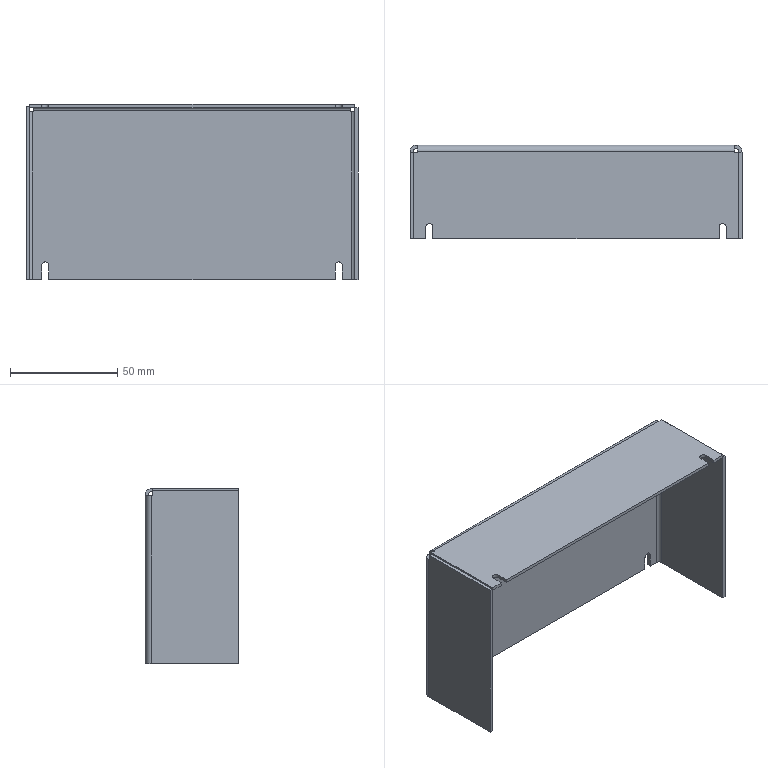Part | STEP file | ROTATION MC_NEW VER-0610_572 | 1 solid | 46 faces | box 154.5 x 43.5 x 81.5 mm | volume 37915 mm3 | plane 36 | cylinder 10 | commonest cylinder face diameters 3.4 x4 3 x3 6 x3
STEP:
#1=CARTESIAN_POINT('',(-189.169,680.758,-56.091));
#2=VERTEX_POINT('',#1);
#3=CARTESIAN_POINT('',(-189.169,680.758,-54.591));
#4=VERTEX_POINT('',#3);
#5=CARTESIAN_POINT('',(-189.169,680.758,-56.091));
#6=DIRECTION('',(0.,0.,1.));
#7=VECTOR('',#6,1.5);
#8=LINE('',#5,#7);
#9=EDGE_CURVE('',#2,#4,#8,.T.);
#10=ORIENTED_EDGE('',*,*,#9,.F.);
#11=CARTESIAN_POINT('',(-185.769,680.758,-56.091));
#12=VERTEX_POINT('',#11);
#13=CARTESIAN_POINT('',(-187.469,680.758,-56.091));
#14=DIRECTION('',(0.,0.,1.));
#15=DIRECTION('',(0.,-1.,0.));
#16=AXIS2_PLACEMENT_3D('',#13,#14,#15);
#17=CIRCLE('',#16,1.7);
#18=EDGE_CURVE('',#12,#2,#17,.T.);
#19=ORIENTED_EDGE('',*,*,#18,.F.);
#20=CARTESIAN_POINT('',(-185.769,680.758,-54.591));
#21=VERTEX_POINT('',#20);
#22=CARTESIAN_POINT('',(-185.769,680.758,-54.591));
#23=DIRECTION('',(0.,0.,-1.));
#24=VECTOR('',#23,1.5);
#25=LINE('',#22,#24);
#26=EDGE_CURVE('',#21,#12,#25,.T.);
#27=ORIENTED_EDGE('',*,*,#26,.F.);
#28=CARTESIAN_POINT('',(-187.469,680.758,-54.591));
#29=DIRECTION('',(0.,0.,-1.));
#30=DIRECTION('',(0.,-1.,0.));
#31=AXIS2_PLACEMENT_3D('',#28,#29,#30);
#32=CIRCLE('',#31,1.7);
#33=EDGE_CURVE('',#4,#21,#32,.T.);
#34=ORIENTED_EDGE('',*,*,#33,.F.);
#35=EDGE_LOOP('',(#10,#19,#27,#34));
#36=FACE_OUTER_BOUND('',#35,.T.);
#37=CARTESIAN_POINT('',(-187.469,680.758,-64.591));
#38=DIRECTION('',(0.,0.,1.));
#39=DIRECTION('',(1.,0.,0.));
#40=AXIS2_PLACEMENT_3D('',#37,#38,#39);
#41=CYLINDRICAL_SURFACE('',#40,1.7);
#42=ADVANCED_FACE('',(#36),#41,.F.);
#43=CARTESIAN_POINT('',(-322.269,680.758,-54.591));
#44=VERTEX_POINT('',#43);
#45=CARTESIAN_POINT('',(-322.269,680.758,-56.091));
#46=VERTEX_POINT('',#45);
#47=CARTESIAN_POINT('',(-322.269,680.758,-54.591));
#48=DIRECTION('',(0.,0.,-1.));
#49=VECTOR('',#48,1.5);
#50=LINE('',#47,#49);
#51=EDGE_CURVE('',#44,#46,#50,.T.);
#52=ORIENTED_EDGE('',*,*,#51,.F.);
#53=CARTESIAN_POINT('',(-325.669,680.758,-54.591));
#54=VERTEX_POINT('',#53);
#55=CARTESIAN_POINT('',(-323.969,680.758,-54.591));
#56=DIRECTION('',(0.,0.,-1.));
#57=DIRECTION('',(0.,-1.,0.));
#58=AXIS2_PLACEMENT_3D('',#55,#56,#57);
#59=CIRCLE('',#58,1.7);
#60=EDGE_CURVE('',#54,#44,#59,.T.);
#61=ORIENTED_EDGE('',*,*,#60,.F.);
#62=CARTESIAN_POINT('',(-325.669,680.758,-56.091));
#63=VERTEX_POINT('',#62);
#64=CARTESIAN_POINT('',(-325.669,680.758,-56.091));
#65=DIRECTION('',(0.,0.,1.));
#66=VECTOR('',#65,1.5);
#67=LINE('',#64,#66);
#68=EDGE_CURVE('',#63,#54,#67,.T.);
#69=ORIENTED_EDGE('',*,*,#68,.F.);
#70=CARTESIAN_POINT('',(-323.969,680.758,-56.091));
#71=DIRECTION('',(0.,0.,1.));
#72=DIRECTION('',(0.,-1.,0.));
#73=AXIS2_PLACEMENT_3D('',#70,#71,#72);
#74=CIRCLE('',#73,1.7);
#75=EDGE_CURVE('',#46,#63,#74,.T.);
#76=ORIENTED_EDGE('',*,*,#75,.F.);
#77=EDGE_LOOP('',(#52,#61,#69,#76));
#78=FACE_OUTER_BOUND('',#77,.T.);
#79=CARTESIAN_POINT('',(-323.969,680.758,-64.591));
#80=DIRECTION('',(0.,0.,1.));
#81=DIRECTION('',(1.,0.,0.));
#82=AXIS2_PLACEMENT_3D('',#79,#80,#81);
#83=CYLINDRICAL_SURFACE('',#82,1.7);
#84=ADVANCED_FACE('',(#78),#83,.F.);
#85=CARTESIAN_POINT('',(-325.669,719.008,-136.091));
#86=VERTEX_POINT('',#85);
#87=CARTESIAN_POINT('',(-325.669,717.508,-136.091));
#88=VERTEX_POINT('',#87);
#89=CARTESIAN_POINT('',(-325.669,719.008,-136.091));
#90=DIRECTION('',(0.,-1.,0.));
#91=VECTOR('',#90,1.5);
#92=LINE('',#89,#91);
#93=EDGE_CURVE('',#86,#88,#92,.T.);
#94=ORIENTED_EDGE('',*,*,#93,.F.);
#95=CARTESIAN_POINT('',(-325.669,719.008,-129.591));
#96=VERTEX_POINT('',#95);
#97=CARTESIAN_POINT('',(-325.669,719.008,-129.591));
#98=DIRECTION('',(0.,0.,-1.));
#99=VECTOR('',#98,6.5);
#100=LINE('',#97,#99);
#101=EDGE_CURVE('',#96,#86,#100,.T.);
#102=ORIENTED_EDGE('',*,*,#101,.F.);
#103=CARTESIAN_POINT('',(-325.669,717.508,-129.591));
#104=VERTEX_POINT('',#103);
#105=CARTESIAN_POINT('',(-325.669,719.008,-129.591));
#106=DIRECTION('',(0.,-1.,0.));
#107=VECTOR('',#106,1.5);
#108=LINE('',#105,#107);
#109=EDGE_CURVE('',#96,#104,#108,.T.);
#110=ORIENTED_EDGE('',*,*,#109,.T.);
#111=CARTESIAN_POINT('',(-325.669,717.508,-136.091));
#112=DIRECTION('',(0.,0.,1.));
#113=VECTOR('',#112,6.5);
#114=LINE('',#111,#113);
#115=EDGE_CURVE('',#88,#104,#114,.T.);
#116=ORIENTED_EDGE('',*,*,#115,.F.);
#117=EDGE_LOOP('',(#94,#102,#110,#116));
#118=FACE_OUTER_BOUND('',#117,.T.);
#119=CARTESIAN_POINT('',(-325.669,719.008,-133.291));
#120=DIRECTION('',(-1.,0.,0.));
#121=DIRECTION('',(0.,0.,1.));
#122=AXIS2_PLACEMENT_3D('',#119,#120,#121);
#123=PLANE('',#122);
#124=ADVANCED_FACE('',(#118),#123,.F.);
#125=ORIENTED_EDGE('',*,*,#101,.T.);
#126=CARTESIAN_POINT('',(-329.969,719.008,-136.091));
#127=VERTEX_POINT('',#126);
#128=CARTESIAN_POINT('',(-329.969,719.008,-136.091));
#129=DIRECTION('',(1.,0.,0.));
#130=VECTOR('',#129,4.3);
#131=LINE('',#128,#130);
#132=EDGE_CURVE('',#127,#86,#131,.T.);
#133=ORIENTED_EDGE('',*,*,#132,.F.);
#134=CARTESIAN_POINT('',(-329.969,719.008,-57.966));
#135=VERTEX_POINT('',#134);
#136=CARTESIAN_POINT('',(-329.969,719.008,-57.966));
#137=DIRECTION('',(0.,0.,-1.));
#138=VECTOR('',#137,78.125);
#139=LINE('',#136,#138);
#140=EDGE_CURVE('',#135,#127,#139,.T.);
#141=ORIENTED_EDGE('',*,*,#140,.F.);
#142=CARTESIAN_POINT('',(-329.594,719.008,-57.966));
#143=VERTEX_POINT('',#142);
#144=CARTESIAN_POINT('',(-329.594,719.008,-57.966));
#145=DIRECTION('',(-1.,0.,0.));
#146=VECTOR('',#145,0.375);
#147=LINE('',#144,#146);
#148=EDGE_CURVE('',#143,#135,#147,.T.);
#149=ORIENTED_EDGE('',*,*,#148,.F.);
#150=CARTESIAN_POINT('',(-329.594,719.008,-57.591));
#151=VERTEX_POINT('',#150);
#152=CARTESIAN_POINT('',(-329.594,719.008,-57.591));
#153=DIRECTION('',(0.,0.,-1.));
#154=VECTOR('',#153,0.375);
#155=LINE('',#152,#154);
#156=EDGE_CURVE('',#151,#143,#155,.T.);
#157=ORIENTED_EDGE('',*,*,#156,.F.);
#158=CARTESIAN_POINT('',(-181.844,719.008,-57.591));
#159=VERTEX_POINT('',#158);
#160=CARTESIAN_POINT('',(-181.844,719.008,-57.591));
#161=DIRECTION('',(-1.,0.,0.));
#162=VECTOR('',#161,147.75);
#163=LINE('',#160,#162);
#164=EDGE_CURVE('',#159,#151,#163,.T.);
#165=ORIENTED_EDGE('',*,*,#164,.F.);
#166=CARTESIAN_POINT('',(-181.844,719.008,-57.966));
#167=VERTEX_POINT('',#166);
#168=CARTESIAN_POINT('',(-181.844,719.008,-57.966));
#169=DIRECTION('',(0.,0.,1.));
#170=VECTOR('',#169,0.375);
#171=LINE('',#168,#170);
#172=EDGE_CURVE('',#167,#159,#171,.T.);
#173=ORIENTED_EDGE('',*,*,#172,.F.);
#174=CARTESIAN_POINT('',(-181.469,719.008,-57.966));
#175=VERTEX_POINT('',#174);
#176=CARTESIAN_POINT('',(-181.469,719.008,-57.966));
#177=DIRECTION('',(-1.,0.,0.));
#178=VECTOR('',#177,0.375);
#179=LINE('',#176,#178);
#180=EDGE_CURVE('',#175,#167,#179,.T.);
#181=ORIENTED_EDGE('',*,*,#180,.F.);
#182=CARTESIAN_POINT('',(-181.469,719.008,-136.091));
#183=VERTEX_POINT('',#182);
#184=CARTESIAN_POINT('',(-181.469,719.008,-136.091));
#185=DIRECTION('',(0.,0.,1.));
#186=VECTOR('',#185,78.125);
#187=LINE('',#184,#186);
#188=EDGE_CURVE('',#183,#175,#187,.T.);
#189=ORIENTED_EDGE('',*,*,#188,.F.);
#190=CARTESIAN_POINT('',(-185.769,719.008,-136.091));
#191=VERTEX_POINT('',#190);
#192=CARTESIAN_POINT('',(-185.769,719.008,-136.091));
#193=DIRECTION('',(1.,0.,0.));
#194=VECTOR('',#193,4.3);
#195=LINE('',#192,#194);
#196=EDGE_CURVE('',#191,#183,#195,.T.);
#197=ORIENTED_EDGE('',*,*,#196,.F.);
#198=CARTESIAN_POINT('',(-185.769,719.008,-129.591));
#199=VERTEX_POINT('',#198);
#200=CARTESIAN_POINT('',(-185.769,719.008,-129.591));
#201=DIRECTION('',(0.,0.,-1.));
#202=VECTOR('',#201,6.5);
#203=LINE('',#200,#202);
#204=EDGE_CURVE('',#199,#191,#203,.T.);
#205=ORIENTED_EDGE('',*,*,#204,.F.);
#206=CARTESIAN_POINT('',(-189.169,719.008,-129.591));
#207=VERTEX_POINT('',#206);
#208=CARTESIAN_POINT('',(-187.469,719.008,-129.591));
#209=DIRECTION('',(0.,-1.,0.));
#210=DIRECTION('',(0.,0.,1.));
#211=AXIS2_PLACEMENT_3D('',#208,#209,#210);
#212=CIRCLE('',#211,1.7);
#213=EDGE_CURVE('',#199,#207,#212,.T.);
#214=ORIENTED_EDGE('',*,*,#213,.T.);
#215=CARTESIAN_POINT('',(-189.169,719.008,-136.091));
#216=VERTEX_POINT('',#215);
#217=CARTESIAN_POINT('',(-189.169,719.008,-136.091));
#218=DIRECTION('',(0.,0.,1.));
#219=VECTOR('',#218,6.5);
#220=LINE('',#217,#219);
#221=EDGE_CURVE('',#216,#207,#220,.T.);
#222=ORIENTED_EDGE('',*,*,#221,.F.);
#223=CARTESIAN_POINT('',(-322.269,719.008,-136.091));
#224=VERTEX_POINT('',#223);
#225=CARTESIAN_POINT('',(-322.269,719.008,-136.091));
#226=DIRECTION('',(1.,0.,0.));
#227=VECTOR('',#226,133.1);
#228=LINE('',#225,#227);
#229=EDGE_CURVE('',#224,#216,#228,.T.);
#230=ORIENTED_EDGE('',*,*,#229,.F.);
#231=CARTESIAN_POINT('',(-322.269,719.008,-129.591));
#232=VERTEX_POINT('',#231);
#233=CARTESIAN_POINT('',(-322.269,719.008,-136.091));
#234=DIRECTION('',(0.,0.,1.));
#235=VECTOR('',#234,6.5);
#236=LINE('',#233,#235);
#237=EDGE_CURVE('',#224,#232,#236,.T.);
#238=ORIENTED_EDGE('',*,*,#237,.T.);
#239=CARTESIAN_POINT('',(-323.969,719.008,-129.591));
#240=DIRECTION('',(0.,1.,0.));
#241=DIRECTION('',(0.,0.,1.));
#242=AXIS2_PLACEMENT_3D('',#239,#240,#241);
#243=CIRCLE('',#242,1.7);
#244=EDGE_CURVE('',#96,#232,#243,.T.);
#245=ORIENTED_EDGE('',*,*,#244,.F.);
#246=EDGE_LOOP('',(#125,#133,#141,#149,#157,#165,#173,#181,#189,#197,#205,#214,#222,#230,#238,#245));
#247=FACE_OUTER_BOUND('',#246,.T.);
#248=CARTESIAN_POINT('',(-257.024,719.008,-56.091));
#249=DIRECTION('',(0.,1.,0.));
#250=DIRECTION('',(0.,0.,1.));
#251=AXIS2_PLACEMENT_3D('',#248,#249,#250);
#252=PLANE('',#251);
#253=ADVANCED_FACE('',(#247),#252,.T.);
#254=CARTESIAN_POINT('',(-329.969,717.508,-136.091));
#255=VERTEX_POINT('',#254);
#256=CARTESIAN_POINT('',(-329.969,717.508,-136.091));
#257=DIRECTION('',(1.,0.,0.));
#258=VECTOR('',#257,4.3);
#259=LINE('',#256,#258);
#260=EDGE_CURVE('',#255,#88,#259,.T.);
#261=ORIENTED_EDGE('',*,*,#260,.T.);
#262=ORIENTED_EDGE('',*,*,#115,.T.);
#263=CARTESIAN_POINT('',(-322.269,717.508,-129.591));
#264=VERTEX_POINT('',#263);
#265=CARTESIAN_POINT('',(-323.969,717.508,-129.591));
#266=DIRECTION('',(0.,1.,0.));
#267=DIRECTION('',(0.,0.,1.));
#268=AXIS2_PLACEMENT_3D('',#265,#266,#267);
#269=CIRCLE('',#268,1.7);
#270=EDGE_CURVE('',#104,#264,#269,.T.);
#271=ORIENTED_EDGE('',*,*,#270,.T.);
#272=CARTESIAN_POINT('',(-322.269,717.508,-136.091));
#273=VERTEX_POINT('',#272);
#274=CARTESIAN_POINT('',(-322.269,717.508,-129.591));
#275=DIRECTION('',(0.,0.,-1.));
#276=VECTOR('',#275,6.5);
#277=LINE('',#274,#276);
#278=EDGE_CURVE('',#264,#273,#277,.T.);
#279=ORIENTED_EDGE('',*,*,#278,.T.);
#280=CARTESIAN_POINT('',(-189.169,717.508,-136.091));
#281=VERTEX_POINT('',#280);
#282=CARTESIAN_POINT('',(-322.269,717.508,-136.091));
#283=DIRECTION('',(1.,0.,0.));
#284=VECTOR('',#283,133.1);
#285=LINE('',#282,#284);
#286=EDGE_CURVE('',#273,#281,#285,.T.);
#287=ORIENTED_EDGE('',*,*,#286,.T.);
#288=CARTESIAN_POINT('',(-189.169,717.508,-129.591));
#289=VERTEX_POINT('',#288);
#290=CARTESIAN_POINT('',(-189.169,717.508,-136.091));
#291=DIRECTION('',(0.,0.,1.));
#292=VECTOR('',#291,6.5);
#293=LINE('',#290,#292);
#294=EDGE_CURVE('',#281,#289,#293,.T.);
#295=ORIENTED_EDGE('',*,*,#294,.T.);
#296=CARTESIAN_POINT('',(-185.769,717.508,-129.591));
#297=VERTEX_POINT('',#296);
#298=CARTESIAN_POINT('',(-187.469,717.508,-129.591));
#299=DIRECTION('',(0.,1.,0.));
#300=DIRECTION('',(0.,0.,1.));
#301=AXIS2_PLACEMENT_3D('',#298,#299,#300);
#302=CIRCLE('',#301,1.7);
#303=EDGE_CURVE('',#289,#297,#302,.T.);
#304=ORIENTED_EDGE('',*,*,#303,.T.);
#305=CARTESIAN_POINT('',(-185.769,717.508,-136.091));
#306=VERTEX_POINT('',#305);
#307=CARTESIAN_POINT('',(-185.769,717.508,-129.591));
#308=DIRECTION('',(0.,0.,-1.));
#309=VECTOR('',#308,6.5);
#310=LINE('',#307,#309);
#311=EDGE_CURVE('',#297,#306,#310,.T.);
#312=ORIENTED_EDGE('',*,*,#311,.T.);
#313=CARTESIAN_POINT('',(-181.469,717.508,-136.091));
#314=VERTEX_POINT('',#313);
#315=CARTESIAN_POINT('',(-185.769,717.508,-136.091));
#316=DIRECTION('',(1.,0.,0.));
#317=VECTOR('',#316,4.3);
#318=LINE('',#315,#317);
#319=EDGE_CURVE('',#306,#314,#318,.T.);
#320=ORIENTED_EDGE('',*,*,#319,.T.);
#321=CARTESIAN_POINT('',(-181.469,717.508,-57.966));
#322=VERTEX_POINT('',#321);
#323=CARTESIAN_POINT('',(-181.469,717.508,-57.966));
#324=DIRECTION('',(0.,0.,-1.));
#325=VECTOR('',#324,78.125);
#326=LINE('',#323,#325);
#327=EDGE_CURVE('',#322,#314,#326,.T.);
#328=ORIENTED_EDGE('',*,*,#327,.F.);
#329=CARTESIAN_POINT('',(-181.844,717.508,-57.966));
#330=VERTEX_POINT('',#329);
#331=CARTESIAN_POINT('',(-181.844,717.508,-57.966));
#332=DIRECTION('',(1.,0.,0.));
#333=VECTOR('',#332,0.375);
#334=LINE('',#331,#333);
#335=EDGE_CURVE('',#330,#322,#334,.T.);
#336=ORIENTED_EDGE('',*,*,#335,.F.);
#337=CARTESIAN_POINT('',(-181.844,717.508,-57.591));
#338=VERTEX_POINT('',#337);
#339=CARTESIAN_POINT('',(-181.844,717.508,-57.591));
#340=DIRECTION('',(0.,0.,-1.));
#341=VECTOR('',#340,0.375);
#342=LINE('',#339,#341);
#343=EDGE_CURVE('',#338,#330,#342,.T.);
#344=ORIENTED_EDGE('',*,*,#343,.F.);
#345=CARTESIAN_POINT('',(-329.594,717.508,-57.591));
#346=VERTEX_POINT('',#345);
#347=CARTESIAN_POINT('',(-329.594,717.508,-57.591));
#348=DIRECTION('',(1.,0.,0.));
#349=VECTOR('',#348,147.75);
#350=LINE('',#347,#349);
#351=EDGE_CURVE('',#346,#338,#350,.T.);
#352=ORIENTED_EDGE('',*,*,#351,.F.);
#353=CARTESIAN_POINT('',(-329.594,717.508,-57.966));
#354=VERTEX_POINT('',#353);
#355=CARTESIAN_POINT('',(-329.594,717.508,-57.966));
#356=DIRECTION('',(0.,0.,1.));
#357=VECTOR('',#356,0.375);
#358=LINE('',#355,#357);
#359=EDGE_CURVE('',#354,#346,#358,.T.);
#360=ORIENTED_EDGE('',*,*,#359,.F.);
#361=CARTESIAN_POINT('',(-329.969,717.508,-57.966));
#362=VERTEX_POINT('',#361);
#363=CARTESIAN_POINT('',(-329.969,717.508,-57.966));
#364=DIRECTION('',(1.,0.,0.));
#365=VECTOR('',#364,0.375);
#366=LINE('',#363,#365);
#367=EDGE_CURVE('',#362,#354,#366,.T.);
#368=ORIENTED_EDGE('',*,*,#367,.F.);
#369=CARTESIAN_POINT('',(-329.969,717.508,-136.091));
#370=DIRECTION('',(0.,0.,1.));
#371=VECTOR('',#370,78.125);
#372=LINE('',#369,#371);
#373=EDGE_CURVE('',#255,#362,#372,.T.);
#374=ORIENTED_EDGE('',*,*,#373,.F.);
#375=EDGE_LOOP('',(#261,#262,#271,#279,#287,#295,#304,#312,#320,#328,#336,#344,#352,#360,#368,#374));
#376=FACE_OUTER_BOUND('',#375,.T.);
#377=CARTESIAN_POINT('',(-121.999,717.508,-143.591));
#378=DIRECTION('',(0.,1.,0.));
#379=DIRECTION('',(0.,0.,1.));
#380=AXIS2_PLACEMENT_3D('',#377,#378,#379);
#381=PLANE('',#380);
#382=ADVANCED_FACE('',(#376),#381,.F.);
#383=ORIENTED_EDGE('',*,*,#132,.T.);
#384=ORIENTED_EDGE('',*,*,#93,.T.);
#385=ORIENTED_EDGE('',*,*,#260,.F.);
#386=CARTESIAN_POINT('',(-331.469,716.008,-136.091));
#387=VERTEX_POINT('',#386);
#388=CARTESIAN_POINT('',(-329.969,716.008,-136.091));
#389=DIRECTION('',(0.,0.,1.));
#390=DIRECTION('',(-0.7071,0.7071,0.));
#391=AXIS2_PLACEMENT_3D('',#388,#389,#390);
#392=CIRCLE('',#391,1.5);
#393=EDGE_CURVE('',#255,#387,#392,.T.);
#394=ORIENTED_EDGE('',*,*,#393,.T.);
#395=CARTESIAN_POINT('',(-331.469,675.508,-136.091));
#396=VERTEX_POINT('',#395);
#397=CARTESIAN_POINT('',(-331.469,716.008,-136.091));
#398=DIRECTION('',(0.,-1.,0.));
#399=VECTOR('',#398,40.5);
#400=LINE('',#397,#399);
#401=EDGE_CURVE('',#387,#396,#400,.T.);
#402=ORIENTED_EDGE('',*,*,#401,.T.);
#403=CARTESIAN_POINT('',(-332.969,675.508,-136.091));
#404=VERTEX_POINT('',#403);
#405=CARTESIAN_POINT('',(-332.969,675.508,-136.091));
#406=DIRECTION('',(1.,0.,0.));
#407=VECTOR('',#406,1.5);
#408=LINE('',#405,#407);
#409=EDGE_CURVE('',#404,#396,#408,.T.);
#410=ORIENTED_EDGE('',*,*,#409,.F.);
#411=CARTESIAN_POINT('',(-332.969,716.008,-136.091));
#412=VERTEX_POINT('',#411);
#413=CARTESIAN_POINT('',(-332.969,716.008,-136.091));
#414=DIRECTION('',(0.,-1.,0.));
#415=VECTOR('',#414,40.5);
#416=LINE('',#413,#415);
#417=EDGE_CURVE('',#412,#404,#416,.T.);
#418=ORIENTED_EDGE('',*,*,#417,.F.);
#419=CARTESIAN_POINT('',(-329.969,716.008,-136.091));
#420=DIRECTION('',(0.,0.,-1.));
#421=DIRECTION('',(-1.,0.,0.));
#422=AXIS2_PLACEMENT_3D('',#419,#420,#421);
#423=CIRCLE('',#422,3.);
#424=EDGE_CURVE('',#412,#127,#423,.T.);
#425=ORIENTED_EDGE('',*,*,#424,.T.);
#426=EDGE_LOOP('',(#383,#384,#385,#394,#402,#410,#418,#425));
#427=FACE_OUTER_BOUND('',#426,.T.);
#428=CARTESIAN_POINT('',(-570.084,581.438,-136.091));
#429=DIRECTION('',(0.,0.,-1.));
#430=DIRECTION('',(-1.,0.,0.));
#431=AXIS2_PLACEMENT_3D('',#428,#429,#430);
#432=PLANE('',#431);
#433=ADVANCED_FACE('',(#427),#432,.T.);
#434=ORIENTED_EDGE('',*,*,#286,.F.);
#435=CARTESIAN_POINT('',(-322.269,717.508,-136.091));
#436=DIRECTION('',(0.,1.,0.));
#437=VECTOR('',#436,1.5);
#438=LINE('',#435,#437);
#439=EDGE_CURVE('',#273,#224,#438,.T.);
#440=ORIENTED_EDGE('',*,*,#439,.T.);
#441=ORIENTED_EDGE('',*,*,#229,.T.);
#442=CARTESIAN_POINT('',(-189.169,719.008,-136.091));
#443=DIRECTION('',(0.,-1.,0.));
#444=VECTOR('',#443,1.5);
#445=LINE('',#442,#444);
#446=EDGE_CURVE('',#216,#281,#445,.T.);
#447=ORIENTED_EDGE('',*,*,#446,.T.);
#448=EDGE_LOOP('',(#434,#440,#441,#447));
#449=FACE_OUTER_BOUND('',#448,.T.);
#450=CARTESIAN_POINT('',(-570.084,581.438,-136.091));
#451=DIRECTION('',(0.,0.,-1.));
#452=DIRECTION('',(-1.,0.,0.));
#453=AXIS2_PLACEMENT_3D('',#450,#451,#452);
#454=PLANE('',#453);
#455=ADVANCED_FACE('',(#449),#454,.T.);
#456=ORIENTED_EDGE('',*,*,#221,.T.);
#457=CARTESIAN_POINT('',(-189.169,719.008,-129.591));
#458=DIRECTION('',(0.,-1.,0.));
#459=VECTOR('',#458,1.5);
#460=LINE('',#457,#459);
#461=EDGE_CURVE('',#207,#289,#460,.T.);
#462=ORIENTED_EDGE('',*,*,#461,.T.);
#463=ORIENTED_EDGE('',*,*,#294,.F.);
#464=ORIENTED_EDGE('',*,*,#446,.F.);
#465=EDGE_LOOP('',(#456,#462,#463,#464));
#466=FACE_OUTER_BOUND('',#465,.T.);
#467=CARTESIAN_POINT('',(-189.169,719.008,-133.291));
#468=DIRECTION('',(-1.,0.,0.));
#469=DIRECTION('',(0.,0.,1.));
#470=AXIS2_PLACEMENT_3D('',#467,#468,#469);
#471=PLANE('',#470);
#472=ADVANCED_FACE('',(#466),#471,.F.);
#473=ORIENTED_EDGE('',*,*,#461,.F.);
#474=ORIENTED_EDGE('',*,*,#213,.F.);
#475=CARTESIAN_POINT('',(-185.769,717.508,-129.591));
#476=DIRECTION('',(0.,1.,0.));
#477=VECTOR('',#476,1.5);
#478=LINE('',#475,#477);
#479=EDGE_CURVE('',#297,#199,#478,.T.);
#480=ORIENTED_EDGE('',*,*,#479,.F.);
#481=ORIENTED_EDGE('',*,*,#303,.F.);
#482=EDGE_LOOP('',(#473,#474,#480,#481));
#483=FACE_OUTER_BOUND('',#482,.T.);
#484=CARTESIAN_POINT('',(-187.469,719.008,-129.591));
#485=DIRECTION('',(0.,1.,0.));
#486=DIRECTION('',(0.,0.,1.));
#487=AXIS2_PLACEMENT_3D('',#484,#485,#486);
#488=CYLINDRICAL_SURFACE('',#487,1.7);
#489=ADVANCED_FACE('',(#483),#488,.F.);
#490=ORIENTED_EDGE('',*,*,#311,.F.);
#491=ORIENTED_EDGE('',*,*,#479,.T.);
#492=ORIENTED_EDGE('',*,*,#204,.T.);
#493=CARTESIAN_POINT('',(-185.769,717.508,-136.091));
#494=DIRECTION('',(0.,1.,0.));
#495=VECTOR('',#494,1.5);
#496=LINE('',#493,#495);
#497=EDGE_CURVE('',#306,#191,#496,.T.);
#498=ORIENTED_EDGE('',*,*,#497,.F.);
#499=EDGE_LOOP('',(#490,#491,#492,#498));
#500=FACE_OUTER_BOUND('',#499,.T.);
#501=CARTESIAN_POINT('',(-185.769,719.008,-133.291));
#502=DIRECTION('',(1.,0.,0.));
#503=DIRECTION('',(0.,0.,-1.));
#504=AXIS2_PLACEMENT_3D('',#501,#502,#503);
#505=PLANE('',#504);
#506=ADVANCED_FACE('',(#500),#505,.F.);
#507=ORIENTED_EDGE('',*,*,#319,.F.);
#508=ORIENTED_EDGE('',*,*,#497,.T.);
#509=ORIENTED_EDGE('',*,*,#196,.T.);
#510=CARTESIAN_POINT('',(-178.469,716.008,-136.091));
#511=VERTEX_POINT('',#510);
#512=CARTESIAN_POINT('',(-181.469,716.008,-136.091));
#513=DIRECTION('',(0.,0.,-1.));
#514=DIRECTION('',(0.,1.,0.));
#515=AXIS2_PLACEMENT_3D('',#512,#513,#514);
#516=CIRCLE('',#515,3.);
#517=EDGE_CURVE('',#183,#511,#516,.T.);
#518=ORIENTED_EDGE('',*,*,#517,.T.);
#519=CARTESIAN_POINT('',(-178.469,675.508,-136.091));
#520=VERTEX_POINT('',#519);
#521=CARTESIAN_POINT('',(-178.469,675.508,-136.091));
#522=DIRECTION('',(0.,1.,0.));
#523=VECTOR('',#522,40.5);
#524=LINE('',#521,#523);
#525=EDGE_CURVE('',#520,#511,#524,.T.);
#526=ORIENTED_EDGE('',*,*,#525,.F.);
#527=CARTESIAN_POINT('',(-179.969,675.508,-136.091));
#528=VERTEX_POINT('',#527);
#529=CARTESIAN_POINT('',(-178.469,675.508,-136.091));
#530=DIRECTION('',(-1.,0.,0.));
#531=VECTOR('',#530,1.5);
#532=LINE('',#529,#531);
#533=EDGE_CURVE('',#520,#528,#532,.T.);
#534=ORIENTED_EDGE('',*,*,#533,.T.);
#535=CARTESIAN_POINT('',(-179.969,716.008,-136.091));
#536=VERTEX_POINT('',#535);
#537=CARTESIAN_POINT('',(-179.969,716.008,-136.091));
#538=DIRECTION('',(0.,-1.,0.));
#539=VECTOR('',#538,40.5);
#540=LINE('',#537,#539);
#541=EDGE_CURVE('',#536,#528,#540,.T.);
#542=ORIENTED_EDGE('',*,*,#541,.F.);
#543=CARTESIAN_POINT('',(-181.469,716.008,-136.091));
#544=DIRECTION('',(0.,0.,1.));
#545=DIRECTION('',(1.,0.,0.));
#546=AXIS2_PLACEMENT_3D('',#543,#544,#545);
#547=CIRCLE('',#546,1.5);
#548=EDGE_CURVE('',#536,#314,#547,.T.);
#549=ORIENTED_EDGE('',*,*,#548,.T.);
#550=EDGE_LOOP('',(#507,#508,#509,#518,#526,#534,#542,#549));
#551=FACE_OUTER_BOUND('',#550,.T.);
#552=CARTESIAN_POINT('',(-570.084,581.438,-136.091));
#553=DIRECTION('',(0.,0.,-1.));
#554=DIRECTION('',(-1.,0.,0.));
#555=AXIS2_PLACEMENT_3D('',#552,#553,#554);
#556=PLANE('',#555);
#557=ADVANCED_FACE('',(#551),#556,.T.);
#558=CARTESIAN_POINT('',(-179.969,716.008,-57.966));
#559=VERTEX_POINT('',#558);
#560=CARTESIAN_POINT('',(-181.469,716.008,-57.966));
#561=DIRECTION('',(0.,0.,-1.));
#562=DIRECTION('',(0.,1.,0.));
#563=AXIS2_PLACEMENT_3D('',#560,#561,#562);
#564=CIRCLE('',#563,1.5);
#565=EDGE_CURVE('',#322,#559,#564,.T.);
#566=ORIENTED_EDGE('',*,*,#565,.F.);
#567=ORIENTED_EDGE('',*,*,#327,.T.);
#568=ORIENTED_EDGE('',*,*,#548,.F.);
#569=CARTESIAN_POINT('',(-179.969,716.008,-136.091));
#570=DIRECTION('',(0.,0.,1.));
#571=VECTOR('',#570,78.125);
#572=LINE('',#569,#571);
#573=EDGE_CURVE('',#536,#559,#572,.T.);
#574=ORIENTED_EDGE('',*,*,#573,.T.);
#575=EDGE_LOOP('',(#566,#567,#568,#574));
#576=FACE_OUTER_BOUND('',#575,.T.);
#577=CARTESIAN_POINT('',(-181.469,716.008,-136.091));
#578=DIRECTION('',(0.,0.,1.));
#579=DIRECTION('',(-1.,0.,0.));
#580=AXIS2_PLACEMENT_3D('',#577,#578,#579);
#581=CYLINDRICAL_SURFACE('',#580,1.5);
#582=ADVANCED_FACE('',(#576),#581,.F.);
#583=ORIENTED_EDGE('',*,*,#335,.T.);
#584=ORIENTED_EDGE('',*,*,#565,.T.);
#585=CARTESIAN_POINT('',(-179.969,715.633,-57.966));
#586=VERTEX_POINT('',#585);
#587=CARTESIAN_POINT('',(-179.969,716.008,-57.966));
#588=DIRECTION('',(0.,-1.,0.));
#589=VECTOR('',#588,0.375);
#590=LINE('',#587,#589);
#591=EDGE_CURVE('',#559,#586,#590,.T.);
#592=ORIENTED_EDGE('',*,*,#591,.T.);
#593=CARTESIAN_POINT('',(-178.469,715.633,-57.966));
#594=VERTEX_POINT('',#593);
#595=CARTESIAN_POINT('',(-178.469,715.633,-57.966));
#596=DIRECTION('',(-1.,0.,0.));
#597=VECTOR('',#596,1.5);
#598=LINE('',#595,#597);
#599=EDGE_CURVE('',#594,#586,#598,.T.);
#600=ORIENTED_EDGE('',*,*,#599,.F.);
#601=CARTESIAN_POINT('',(-178.469,716.008,-57.966));
#602=VERTEX_POINT('',#601);
#603=CARTESIAN_POINT('',(-178.469,715.633,-57.966));
#604=DIRECTION('',(0.,1.,0.));
#605=VECTOR('',#604,0.375);
#606=LINE('',#603,#605);
#607=EDGE_CURVE('',#594,#602,#606,.T.);
#608=ORIENTED_EDGE('',*,*,#607,.T.);
#609=CARTESIAN_POINT('',(-181.469,716.008,-57.966));
#610=DIRECTION('',(0.,0.,1.));
#611=DIRECTION('',(1.,0.,0.));
#612=AXIS2_PLACEMENT_3D('',#609,#610,#611);
#613=CIRCLE('',#612,3.);
#614=EDGE_CURVE('',#602,#175,#613,.T.);
#615=ORIENTED_EDGE('',*,*,#614,.T.);
#616=ORIENTED_EDGE('',*,*,#180,.T.);
#617=CARTESIAN_POINT('',(-181.844,719.008,-57.966));
#618=DIRECTION('',(0.,-1.,0.));
#619=VECTOR('',#618,1.5);
#620=LINE('',#617,#619);
#621=EDGE_CURVE('',#167,#330,#620,.T.);
#622=ORIENTED_EDGE('',*,*,#621,.T.);
#623=EDGE_LOOP('',(#583,#584,#592,#600,#608,#615,#616,#622));
#624=FACE_OUTER_BOUND('',#623,.T.);
#625=CARTESIAN_POINT('',(-178.469,717.321,-57.966));
#626=DIRECTION('',(0.,0.,-1.));
#627=DIRECTION('',(-1.,0.,0.));
#628=AXIS2_PLACEMENT_3D('',#625,#626,#627);
#629=PLANE('',#628);
#630=ADVANCED_FACE('',(#624),#629,.F.);
#631=CARTESIAN_POINT('',(-181.844,715.633,-56.091));
#632=VERTEX_POINT('',#631);
#633=CARTESIAN_POINT('',(-181.844,716.008,-56.091));
#634=VERTEX_POINT('',#633);
#635=CARTESIAN_POINT('',(-181.844,715.633,-56.091));
#636=DIRECTION('',(0.,1.,0.));
#637=VECTOR('',#636,0.375);
#638=LINE('',#635,#637);
#639=EDGE_CURVE('',#632,#634,#638,.T.);
#640=ORIENTED_EDGE('',*,*,#639,.T.);
#641=CARTESIAN_POINT('',(-181.844,716.008,-57.591));
#642=DIRECTION('',(-1.,0.,0.));
#643=DIRECTION('',(0.,0.,1.));
#644=AXIS2_PLACEMENT_3D('',#641,#642,#643);
#645=CIRCLE('',#644,1.5);
#646=EDGE_CURVE('',#634,#338,#645,.T.);
#647=ORIENTED_EDGE('',*,*,#646,.T.);
#648=ORIENTED_EDGE('',*,*,#343,.T.);
#649=ORIENTED_EDGE('',*,*,#621,.F.);
#650=ORIENTED_EDGE('',*,*,#172,.T.);
#651=CARTESIAN_POINT('',(-181.844,716.008,-54.591));
#652=VERTEX_POINT('',#651);
#653=CARTESIAN_POINT('',(-181.844,716.008,-57.591));
#654=DIRECTION('',(1.,0.,0.));
#655=DIRECTION('',(0.,1.,0.));
#656=AXIS2_PLACEMENT_3D('',#653,#654,#655);
#657=CIRCLE('',#656,3.);
#658=EDGE_CURVE('',#159,#652,#657,.T.);
#659=ORIENTED_EDGE('',*,*,#658,.T.);
#660=CARTESIAN_POINT('',(-181.844,715.633,-54.591));
#661=VERTEX_POINT('',#660);
#662=CARTESIAN_POINT('',(-181.844,716.008,-54.591));
#663=DIRECTION('',(0.,-1.,0.));
#664=VECTOR('',#663,0.375);
#665=LINE('',#662,#664);
#666=EDGE_CURVE('',#652,#661,#665,.T.);
#667=ORIENTED_EDGE('',*,*,#666,.T.);
#668=CARTESIAN_POINT('',(-181.844,715.633,-54.591));
#669=DIRECTION('',(0.,0.,-1.));
#670=VECTOR('',#669,1.5);
#671=LINE('',#668,#670);
#672=EDGE_CURVE('',#661,#632,#671,.T.);
#673=ORIENTED_EDGE('',*,*,#672,.T.);
#674=EDGE_LOOP('',(#640,#647,#648,#649,#650,#659,#667,#673));
#675=FACE_OUTER_BOUND('',#674,.T.);
#676=CARTESIAN_POINT('',(-181.844,717.321,-54.591));
#677=DIRECTION('',(-1.,0.,0.));
#678=DIRECTION('',(0.,0.,1.));
#679=AXIS2_PLACEMENT_3D('',#676,#677,#678);
#680=PLANE('',#679);
#681=ADVANCED_FACE('',(#675),#680,.F.);
#682=ORIENTED_EDGE('',*,*,#646,.F.);
#683=CARTESIAN_POINT('',(-329.594,716.008,-56.091));
#684=VERTEX_POINT('',#683);
#685=CARTESIAN_POINT('',(-181.844,716.008,-56.091));
#686=DIRECTION('',(-1.,0.,0.));
#687=VECTOR('',#686,147.75);
#688=LINE('',#685,#687);
#689=EDGE_CURVE('',#634,#684,#688,.T.);
#690=ORIENTED_EDGE('',*,*,#689,.T.);
#691=CARTESIAN_POINT('',(-329.594,716.008,-57.591));
#692=DIRECTION('',(1.,0.,0.));
#693=DIRECTION('',(0.,1.,0.));
#694=AXIS2_PLACEMENT_3D('',#691,#692,#693);
#695=CIRCLE('',#694,1.5);
#696=EDGE_CURVE('',#346,#684,#695,.T.);
#697=ORIENTED_EDGE('',*,*,#696,.F.);
#698=ORIENTED_EDGE('',*,*,#351,.T.);
#699=EDGE_LOOP('',(#682,#690,#697,#698));
#700=FACE_OUTER_BOUND('',#699,.T.);
#701=CARTESIAN_POINT('',(-332.994,716.008,-57.591));
#702=DIRECTION('',(1.,0.,0.));
#703=DIRECTION('',(0.,-1.,0.));
#704=AXIS2_PLACEMENT_3D('',#701,#702,#703);
#705=CYLINDRICAL_SURFACE('',#704,1.5);
#706=ADVANCED_FACE('',(#700),#705,.F.);
#707=CARTESIAN_POINT('',(-329.594,715.633,-54.591));
#708=VERTEX_POINT('',#707);
#709=CARTESIAN_POINT('',(-329.594,716.008,-54.591));
#710=VERTEX_POINT('',#709);
#711=CARTESIAN_POINT('',(-329.594,715.633,-54.591));
#712=DIRECTION('',(0.,1.,0.));
#713=VECTOR('',#712,0.375);
#714=LINE('',#711,#713);
#715=EDGE_CURVE('',#708,#710,#714,.T.);
#716=ORIENTED_EDGE('',*,*,#715,.T.);
#717=CARTESIAN_POINT('',(-329.594,716.008,-57.591));
#718=DIRECTION('',(-1.,0.,0.));
#719=DIRECTION('',(0.,0.,1.));
#720=AXIS2_PLACEMENT_3D('',#717,#718,#719);
#721=CIRCLE('',#720,3.);
#722=EDGE_CURVE('',#710,#151,#721,.T.);
#723=ORIENTED_EDGE('',*,*,#722,.T.);
#724=ORIENTED_EDGE('',*,*,#156,.T.);
#725=CARTESIAN_POINT('',(-329.594,719.008,-57.966));
#726=DIRECTION('',(0.,-1.,0.));
#727=VECTOR('',#726,1.5);
#728=LINE('',#725,#727);
#729=EDGE_CURVE('',#143,#354,#728,.T.);
#730=ORIENTED_EDGE('',*,*,#729,.T.);
#731=ORIENTED_EDGE('',*,*,#359,.T.);
#732=ORIENTED_EDGE('',*,*,#696,.T.);
#733=CARTESIAN_POINT('',(-329.594,715.633,-56.091));
#734=VERTEX_POINT('',#733);
#735=CARTESIAN_POINT('',(-329.594,716.008,-56.091));
#736=DIRECTION('',(0.,-1.,0.));
#737=VECTOR('',#736,0.375);
#738=LINE('',#735,#737);
#739=EDGE_CURVE('',#684,#734,#738,.T.);
#740=ORIENTED_EDGE('',*,*,#739,.T.);
#741=CARTESIAN_POINT('',(-329.594,715.633,-54.591));
#742=DIRECTION('',(0.,0.,-1.));
#743=VECTOR('',#742,1.5);
#744=LINE('',#741,#743);
#745=EDGE_CURVE('',#708,#734,#744,.T.);
#746=ORIENTED_EDGE('',*,*,#745,.F.);
#747=EDGE_LOOP('',(#716,#723,#724,#730,#731,#732,#740,#746));
#748=FACE_OUTER_BOUND('',#747,.T.);
#749=CARTESIAN_POINT('',(-329.594,719.008,-56.279));
#750=DIRECTION('',(1.,0.,0.));
#751=DIRECTION('',(0.,0.,-1.));
#752=AXIS2_PLACEMENT_3D('',#749,#750,#751);
#753=PLANE('',#752);
#754=ADVANCED_FACE('',(#748),#753,.F.);
#755=CARTESIAN_POINT('',(-332.969,716.008,-57.966));
#756=VERTEX_POINT('',#755);
#757=CARTESIAN_POINT('',(-329.969,716.008,-57.966));
#758=DIRECTION('',(0.,0.,1.));
#759=DIRECTION('',(-0.7071,0.7071,0.));
#760=AXIS2_PLACEMENT_3D('',#757,#758,#759);
#761=CIRCLE('',#760,3.);
#762=EDGE_CURVE('',#135,#756,#761,.T.);
#763=ORIENTED_EDGE('',*,*,#762,.T.);
#764=CARTESIAN_POINT('',(-332.969,715.633,-57.966));
#765=VERTEX_POINT('',#764);
#766=CARTESIAN_POINT('',(-332.969,716.008,-57.966));
#767=DIRECTION('',(0.,-1.,0.));
#768=VECTOR('',#767,0.375);
#769=LINE('',#766,#768);
#770=EDGE_CURVE('',#756,#765,#769,.T.);
#771=ORIENTED_EDGE('',*,*,#770,.T.);
#772=CARTESIAN_POINT('',(-331.469,715.633,-57.966));
#773=VERTEX_POINT('',#772);
#774=CARTESIAN_POINT('',(-332.969,715.633,-57.966));
#775=DIRECTION('',(1.,0.,0.));
#776=VECTOR('',#775,1.5);
#777=LINE('',#774,#776);
#778=EDGE_CURVE('',#765,#773,#777,.T.);
#779=ORIENTED_EDGE('',*,*,#778,.T.);
#780=CARTESIAN_POINT('',(-331.469,716.008,-57.966));
#781=VERTEX_POINT('',#780);
#782=CARTESIAN_POINT('',(-331.469,715.633,-57.966));
#783=DIRECTION('',(0.,1.,0.));
#784=VECTOR('',#783,0.375);
#785=LINE('',#782,#784);
#786=EDGE_CURVE('',#773,#781,#785,.T.);
#787=ORIENTED_EDGE('',*,*,#786,.T.);
#788=CARTESIAN_POINT('',(-329.969,716.008,-57.966));
#789=DIRECTION('',(0.,0.,-1.));
#790=DIRECTION('',(-1.,0.,0.));
#791=AXIS2_PLACEMENT_3D('',#788,#789,#790);
#792=CIRCLE('',#791,1.5);
#793=EDGE_CURVE('',#781,#362,#792,.T.);
#794=ORIENTED_EDGE('',*,*,#793,.T.);
#795=ORIENTED_EDGE('',*,*,#367,.T.);
#796=ORIENTED_EDGE('',*,*,#729,.F.);
#797=ORIENTED_EDGE('',*,*,#148,.T.);
#798=EDGE_LOOP('',(#763,#771,#779,#787,#794,#795,#796,#797));
#799=FACE_OUTER_BOUND('',#798,.T.);
#800=CARTESIAN_POINT('',(-336.69,717.321,-57.966));
#801=DIRECTION('',(0.,0.,-1.));
#802=DIRECTION('',(-1.,0.,0.));
#803=AXIS2_PLACEMENT_3D('',#800,#801,#802);
#804=PLANE('',#803);
#805=ADVANCED_FACE('',(#799),#804,.F.);
#806=ORIENTED_EDGE('',*,*,#793,.F.);
#807=CARTESIAN_POINT('',(-331.469,716.008,-57.966));
#808=DIRECTION('',(0.,0.,-1.));
#809=VECTOR('',#808,78.125);
#810=LINE('',#807,#809);
#811=EDGE_CURVE('',#781,#387,#810,.T.);
#812=ORIENTED_EDGE('',*,*,#811,.T.);
#813=ORIENTED_EDGE('',*,*,#393,.F.);
#814=ORIENTED_EDGE('',*,*,#373,.T.);
#815=EDGE_LOOP('',(#806,#812,#813,#814));
#816=FACE_OUTER_BOUND('',#815,.T.);
#817=CARTESIAN_POINT('',(-329.969,716.008,-99.841));
#818=DIRECTION('',(0.,0.,-1.));
#819=DIRECTION('',(-0.7071,0.7071,0.));
#820=AXIS2_PLACEMENT_3D('',#817,#818,#819);
#821=CYLINDRICAL_SURFACE('',#820,1.5);
#822=ADVANCED_FACE('',(#816),#821,.F.);
#823=ORIENTED_EDGE('',*,*,#762,.F.);
#824=ORIENTED_EDGE('',*,*,#140,.T.);
#825=ORIENTED_EDGE('',*,*,#424,.F.);
#826=CARTESIAN_POINT('',(-332.969,716.008,-136.091));
#827=DIRECTION('',(0.,0.,1.));
#828=VECTOR('',#827,78.125);
#829=LINE('',#826,#828);
#830=EDGE_CURVE('',#412,#756,#829,.T.);
#831=ORIENTED_EDGE('',*,*,#830,.T.);
#832=EDGE_LOOP('',(#823,#824,#825,#831));
#833=FACE_OUTER_BOUND('',#832,.T.);
#834=CARTESIAN_POINT('',(-329.969,716.008,-56.091));
#835=DIRECTION('',(0.,0.,-1.));
#836=DIRECTION('',(-0.7071,0.7071,0.));
#837=AXIS2_PLACEMENT_3D('',#834,#835,#836);
#838=CYLINDRICAL_SURFACE('',#837,3.);
#839=ADVANCED_FACE('',(#833),#838,.T.);
#840=ORIENTED_EDGE('',*,*,#658,.F.);
#841=ORIENTED_EDGE('',*,*,#164,.T.);
#842=ORIENTED_EDGE('',*,*,#722,.F.);
#843=CARTESIAN_POINT('',(-329.594,716.008,-54.591));
#844=DIRECTION('',(1.,0.,0.));
#845=VECTOR('',#844,147.75);
#846=LINE('',#843,#845);
#847=EDGE_CURVE('',#710,#652,#846,.T.);
#848=ORIENTED_EDGE('',*,*,#847,.T.);
#849=EDGE_LOOP('',(#840,#841,#842,#848));
#850=FACE_OUTER_BOUND('',#849,.T.);
#851=CARTESIAN_POINT('',(-332.994,716.008,-57.591));
#852=DIRECTION('',(1.,0.,0.));
#853=DIRECTION('',(0.,0.,-1.));
#854=AXIS2_PLACEMENT_3D('',#851,#852,#853);
#855=CYLINDRICAL_SURFACE('',#854,3.);
#856=ADVANCED_FACE('',(#850),#855,.T.);
#857=ORIENTED_EDGE('',*,*,#614,.F.);
#858=CARTESIAN_POINT('',(-178.469,716.008,-57.966));
#859=DIRECTION('',(0.,0.,-1.));
#860=VECTOR('',#859,78.125);
#861=LINE('',#858,#860);
#862=EDGE_CURVE('',#602,#511,#861,.T.);
#863=ORIENTED_EDGE('',*,*,#862,.T.);
#864=ORIENTED_EDGE('',*,*,#517,.F.);
#865=ORIENTED_EDGE('',*,*,#188,.T.);
#866=EDGE_LOOP('',(#857,#863,#864,#865));
#867=FACE_OUTER_BOUND('',#866,.T.);
#868=CARTESIAN_POINT('',(-181.469,716.008,-136.091));
#869=DIRECTION('',(0.,0.,1.));
#870=DIRECTION('',(0.,-1.,0.));
#871=AXIS2_PLACEMENT_3D('',#868,#869,#870);
#872=CYLINDRICAL_SURFACE('',#871,3.);
#873=ADVANCED_FACE('',(#867),#872,.T.);
#874=ORIENTED_EDGE('',*,*,#811,.F.);
#875=ORIENTED_EDGE('',*,*,#786,.F.);
#876=CARTESIAN_POINT('',(-331.469,715.633,-55.341));
#877=VERTEX_POINT('',#876);
#878=CARTESIAN_POINT('',(-331.469,715.633,-55.341));
#879=DIRECTION('',(0.,0.,-1.));
#880=VECTOR('',#879,2.625);
#881=LINE('',#878,#880);
#882=EDGE_CURVE('',#877,#773,#881,.T.);
#883=ORIENTED_EDGE('',*,*,#882,.F.);
#884=CARTESIAN_POINT('',(-331.469,675.508,-55.341));
#885=VERTEX_POINT('',#884);
#886=CARTESIAN_POINT('',(-331.469,715.633,-55.341));
#887=DIRECTION('',(0.,-1.,0.));
#888=VECTOR('',#887,40.125);
#889=LINE('',#886,#888);
#890=EDGE_CURVE('',#877,#885,#889,.T.);
#891=ORIENTED_EDGE('',*,*,#890,.T.);
#892=CARTESIAN_POINT('',(-331.469,675.508,-55.341));
#893=DIRECTION('',(0.,0.,-1.));
#894=VECTOR('',#893,80.75);
#895=LINE('',#892,#894);
#896=EDGE_CURVE('',#885,#396,#895,.T.);
#897=ORIENTED_EDGE('',*,*,#896,.T.);
#898=ORIENTED_EDGE('',*,*,#401,.F.);
#899=EDGE_LOOP('',(#874,#875,#883,#891,#897,#898));
#900=FACE_OUTER_BOUND('',#899,.T.);
#901=CARTESIAN_POINT('',(-331.469,690.623,-56.091));
#902=DIRECTION('',(-1.,0.,0.));
#903=DIRECTION('',(0.,0.,1.));
#904=AXIS2_PLACEMENT_3D('',#901,#902,#903);
#905=PLANE('',#904);
#906=ADVANCED_FACE('',(#900),#905,.F.);
#907=CARTESIAN_POINT('',(-332.969,675.508,-55.341));
#908=VERTEX_POINT('',#907);
#909=CARTESIAN_POINT('',(-331.469,675.508,-55.341));
#910=DIRECTION('',(-1.,0.,0.));
#911=VECTOR('',#910,1.5);
#912=LINE('',#909,#911);
#913=EDGE_CURVE('',#885,#908,#912,.T.);
#914=ORIENTED_EDGE('',*,*,#913,.T.);
#915=CARTESIAN_POINT('',(-332.969,675.508,-136.091));
#916=DIRECTION('',(0.,0.,1.));
#917=VECTOR('',#916,80.75);
#918=LINE('',#915,#917);
#919=EDGE_CURVE('',#404,#908,#918,.T.);
#920=ORIENTED_EDGE('',*,*,#919,.F.);
#921=ORIENTED_EDGE('',*,*,#409,.T.);
#922=ORIENTED_EDGE('',*,*,#896,.F.);
#923=EDGE_LOOP('',(#914,#920,#921,#922));
#924=FACE_OUTER_BOUND('',#923,.T.);
#925=CARTESIAN_POINT('',(-257.344,675.508,-56.091));
#926=DIRECTION('',(0.,-1.,0.));
#927=DIRECTION('',(0.,0.,-1.));
#928=AXIS2_PLACEMENT_3D('',#925,#926,#927);
#929=PLANE('',#928);
#930=ADVANCED_FACE('',(#924),#929,.T.);
#931=ORIENTED_EDGE('',*,*,#830,.F.);
#932=ORIENTED_EDGE('',*,*,#417,.T.);
#933=ORIENTED_EDGE('',*,*,#919,.T.);
#934=CARTESIAN_POINT('',(-332.969,715.633,-55.341));
#935=VERTEX_POINT('',#934);
#936=CARTESIAN_POINT('',(-332.969,675.508,-55.341));
#937=DIRECTION('',(0.,1.,0.));
#938=VECTOR('',#937,40.125);
#939=LINE('',#936,#938);
#940=EDGE_CURVE('',#908,#935,#939,.T.);
#941=ORIENTED_EDGE('',*,*,#940,.T.);
#942=CARTESIAN_POINT('',(-332.969,715.633,-57.966));
#943=DIRECTION('',(0.,0.,1.));
#944=VECTOR('',#943,2.625);
#945=LINE('',#942,#944);
#946=EDGE_CURVE('',#765,#935,#945,.T.);
#947=ORIENTED_EDGE('',*,*,#946,.F.);
#948=ORIENTED_EDGE('',*,*,#770,.F.);
#949=EDGE_LOOP('',(#931,#932,#933,#941,#947,#948));
#950=FACE_OUTER_BOUND('',#949,.T.);
#951=CARTESIAN_POINT('',(-332.969,690.623,-56.091));
#952=DIRECTION('',(-1.,0.,0.));
#953=DIRECTION('',(0.,0.,1.));
#954=AXIS2_PLACEMENT_3D('',#951,#952,#953);
#955=PLANE('',#954);
#956=ADVANCED_FACE('',(#950),#955,.T.);
#957=CARTESIAN_POINT('',(-178.469,715.633,-56.091));
#958=VERTEX_POINT('',#957);
#959=CARTESIAN_POINT('',(-178.469,675.508,-56.091));
#960=VERTEX_POINT('',#959);
#961=CARTESIAN_POINT('',(-178.469,715.633,-56.091));
#962=DIRECTION('',(0.,-1.,0.));
#963=VECTOR('',#962,40.125);
#964=LINE('',#961,#963);
#965=EDGE_CURVE('',#958,#960,#964,.T.);
#966=ORIENTED_EDGE('',*,*,#965,.T.);
#967=CARTESIAN_POINT('',(-178.469,675.508,-56.091));
#968=DIRECTION('',(0.,0.,-1.));
#969=VECTOR('',#968,80.);
#970=LINE('',#967,#969);
#971=EDGE_CURVE('',#960,#520,#970,.T.);
#972=ORIENTED_EDGE('',*,*,#971,.T.);
#973=ORIENTED_EDGE('',*,*,#525,.T.);
#974=ORIENTED_EDGE('',*,*,#862,.F.);
#975=ORIENTED_EDGE('',*,*,#607,.F.);
#976=CARTESIAN_POINT('',(-178.469,715.633,-56.091));
#977=DIRECTION('',(0.,0.,-1.));
#978=VECTOR('',#977,1.875);
#979=LINE('',#976,#978);
#980=EDGE_CURVE('',#958,#594,#979,.T.);
#981=ORIENTED_EDGE('',*,*,#980,.F.);
#982=EDGE_LOOP('',(#966,#972,#973,#974,#975,#981));
#983=FACE_OUTER_BOUND('',#982,.T.);
#984=CARTESIAN_POINT('',(-178.469,690.623,-56.091));
#985=DIRECTION('',(1.,0.,0.));
#986=DIRECTION('',(0.,0.,-1.));
#987=AXIS2_PLACEMENT_3D('',#984,#985,#986);
#988=PLANE('',#987);
#989=ADVANCED_FACE('',(#983),#988,.T.);
#990=CARTESIAN_POINT('',(-179.969,675.508,-56.091));
#991=VERTEX_POINT('',#990);
#992=CARTESIAN_POINT('',(-178.469,675.508,-56.091));
#993=DIRECTION('',(-1.,0.,0.));
#994=VECTOR('',#993,1.5);
#995=LINE('',#992,#994);
#996=EDGE_CURVE('',#960,#991,#995,.T.);
#997=ORIENTED_EDGE('',*,*,#996,.T.);
#998=CARTESIAN_POINT('',(-179.969,675.508,-136.091));
#999=DIRECTION('',(0.,0.,1.));
#1000=VECTOR('',#999,80.);
#1001=LINE('',#998,#1000);
#1002=EDGE_CURVE('',#528,#991,#1001,.T.);
#1003=ORIENTED_EDGE('',*,*,#1002,.F.);
#1004=ORIENTED_EDGE('',*,*,#533,.F.);
#1005=ORIENTED_EDGE('',*,*,#971,.F.);
#1006=EDGE_LOOP('',(#997,#1003,#1004,#1005));
#1007=FACE_OUTER_BOUND('',#1006,.T.);
#1008=CARTESIAN_POINT('',(-256.624,675.508,-56.091));
#1009=DIRECTION('',(0.,-1.,0.));
#1010=DIRECTION('',(0.,0.,-1.));
#1011=AXIS2_PLACEMENT_3D('',#1008,#1009,#1010);
#1012=PLANE('',#1011);
#1013=ADVANCED_FACE('',(#1007),#1012,.T.);
#1014=CARTESIAN_POINT('',(-179.969,715.633,-56.091));
#1015=VERTEX_POINT('',#1014);
#1016=CARTESIAN_POINT('',(-179.969,675.508,-56.091));
#1017=DIRECTION('',(0.,1.,0.));
#1018=VECTOR('',#1017,40.125);
#1019=LINE('',#1016,#1018);
#1020=EDGE_CURVE('',#991,#1015,#1019,.T.);
#1021=ORIENTED_EDGE('',*,*,#1020,.T.);
#1022=CARTESIAN_POINT('',(-179.969,715.633,-57.966));
#1023=DIRECTION('',(0.,0.,1.));
#1024=VECTOR('',#1023,1.875);
#1025=LINE('',#1022,#1024);
#1026=EDGE_CURVE('',#586,#1015,#1025,.T.);
#1027=ORIENTED_EDGE('',*,*,#1026,.F.);
#1028=ORIENTED_EDGE('',*,*,#591,.F.);
#1029=ORIENTED_EDGE('',*,*,#573,.F.);
#1030=ORIENTED_EDGE('',*,*,#541,.T.);
#1031=ORIENTED_EDGE('',*,*,#1002,.T.);
#1032=EDGE_LOOP('',(#1021,#1027,#1028,#1029,#1030,#1031));
#1033=FACE_OUTER_BOUND('',#1032,.T.);
#1034=CARTESIAN_POINT('',(-179.969,690.623,-56.091));
#1035=DIRECTION('',(1.,0.,0.));
#1036=DIRECTION('',(0.,0.,-1.));
#1037=AXIS2_PLACEMENT_3D('',#1034,#1035,#1036);
#1038=PLANE('',#1037);
#1039=ADVANCED_FACE('',(#1033),#1038,.F.);
#1040=CARTESIAN_POINT('',(-179.969,715.633,-56.091));
#1041=DIRECTION('',(1.,0.,0.));
#1042=VECTOR('',#1041,1.5);
#1043=LINE('',#1040,#1042);
#1044=EDGE_CURVE('',#1015,#958,#1043,.T.);
#1045=ORIENTED_EDGE('',*,*,#1044,.T.);
#1046=ORIENTED_EDGE('',*,*,#980,.T.);
#1047=ORIENTED_EDGE('',*,*,#599,.T.);
#1048=ORIENTED_EDGE('',*,*,#1026,.T.);
#1049=EDGE_LOOP('',(#1045,#1046,#1047,#1048));
#1050=FACE_OUTER_BOUND('',#1049,.T.);
#1051=CARTESIAN_POINT('',(-178.469,715.633,-56.279));
#1052=DIRECTION('',(0.,-1.,0.));
#1053=DIRECTION('',(0.,0.,-1.));
#1054=AXIS2_PLACEMENT_3D('',#1051,#1052,#1053);
#1055=PLANE('',#1054);
#1056=ADVANCED_FACE('',(#1050),#1055,.F.);
#1057=CARTESIAN_POINT('',(-322.269,675.508,-56.091));
#1058=VERTEX_POINT('',#1057);
#1059=CARTESIAN_POINT('',(-322.269,675.508,-56.091));
#1060=DIRECTION('',(0.,1.,0.));
#1061=VECTOR('',#1060,5.25);
#1062=LINE('',#1059,#1061);
#1063=EDGE_CURVE('',#1058,#46,#1062,.T.);
#1064=ORIENTED_EDGE('',*,*,#1063,.T.);
#1065=ORIENTED_EDGE('',*,*,#75,.T.);
#1066=CARTESIAN_POINT('',(-325.669,675.508,-56.091));
#1067=VERTEX_POINT('',#1066);
#1068=CARTESIAN_POINT('',(-325.669,680.758,-56.091));
#1069=DIRECTION('',(0.,-1.,0.));
#1070=VECTOR('',#1069,5.25);
#1071=LINE('',#1068,#1070);
#1072=EDGE_CURVE('',#63,#1067,#1071,.T.);
#1073=ORIENTED_EDGE('',*,*,#1072,.T.);
#1074=CARTESIAN_POINT('',(-331.469,675.508,-56.091));
#1075=VERTEX_POINT('',#1074);
#1076=CARTESIAN_POINT('',(-325.669,675.508,-56.091));
#1077=DIRECTION('',(-1.,0.,0.));
#1078=VECTOR('',#1077,5.8);
#1079=LINE('',#1076,#1078);
#1080=EDGE_CURVE('',#1067,#1075,#1079,.T.);
#1081=ORIENTED_EDGE('',*,*,#1080,.T.);
#1082=CARTESIAN_POINT('',(-331.469,715.633,-56.091));
#1083=VERTEX_POINT('',#1082);
#1084=CARTESIAN_POINT('',(-331.469,675.508,-56.091));
#1085=DIRECTION('',(0.,1.,0.));
#1086=VECTOR('',#1085,40.125);
#1087=LINE('',#1084,#1086);
#1088=EDGE_CURVE('',#1075,#1083,#1087,.T.);
#1089=ORIENTED_EDGE('',*,*,#1088,.T.);
#1090=CARTESIAN_POINT('',(-329.594,715.633,-56.091));
#1091=DIRECTION('',(-1.,0.,0.));
#1092=VECTOR('',#1091,1.875);
#1093=LINE('',#1090,#1092);
#1094=EDGE_CURVE('',#734,#1083,#1093,.T.);
#1095=ORIENTED_EDGE('',*,*,#1094,.F.);
#1096=ORIENTED_EDGE('',*,*,#739,.F.);
#1097=ORIENTED_EDGE('',*,*,#689,.F.);
#1098=ORIENTED_EDGE('',*,*,#639,.F.);
#1099=CARTESIAN_POINT('',(-179.969,715.633,-56.091));
#1100=VERTEX_POINT('',#1099);
#1101=CARTESIAN_POINT('',(-179.969,715.633,-56.091));
#1102=DIRECTION('',(-1.,0.,0.));
#1103=VECTOR('',#1102,1.875);
#1104=LINE('',#1101,#1103);
#1105=EDGE_CURVE('',#1100,#632,#1104,.T.);
#1106=ORIENTED_EDGE('',*,*,#1105,.F.);
#1107=CARTESIAN_POINT('',(-179.969,675.508,-56.091));
#1108=VERTEX_POINT('',#1107);
#1109=CARTESIAN_POINT('',(-179.969,715.633,-56.091));
#1110=DIRECTION('',(0.,-1.,0.));
#1111=VECTOR('',#1110,40.125);
#1112=LINE('',#1109,#1111);
#1113=EDGE_CURVE('',#1100,#1108,#1112,.T.);
#1114=ORIENTED_EDGE('',*,*,#1113,.T.);
#1115=CARTESIAN_POINT('',(-185.769,675.508,-56.091));
#1116=VERTEX_POINT('',#1115);
#1117=CARTESIAN_POINT('',(-179.969,675.508,-56.091));
#1118=DIRECTION('',(-1.,0.,0.));
#1119=VECTOR('',#1118,5.8);
#1120=LINE('',#1117,#1119);
#1121=EDGE_CURVE('',#1108,#1116,#1120,.T.);
#1122=ORIENTED_EDGE('',*,*,#1121,.T.);
#1123=CARTESIAN_POINT('',(-185.769,675.508,-56.091));
#1124=DIRECTION('',(0.,1.,0.));
#1125=VECTOR('',#1124,5.25);
#1126=LINE('',#1123,#1125);
#1127=EDGE_CURVE('',#1116,#12,#1126,.T.);
#1128=ORIENTED_EDGE('',*,*,#1127,.T.);
#1129=ORIENTED_EDGE('',*,*,#18,.T.);
#1130=CARTESIAN_POINT('',(-189.169,675.508,-56.091));
#1131=VERTEX_POINT('',#1130);
#1132=CARTESIAN_POINT('',(-189.169,680.758,-56.091));
#1133=DIRECTION('',(0.,-1.,0.));
#1134=VECTOR('',#1133,5.25);
#1135=LINE('',#1132,#1134);
#1136=EDGE_CURVE('',#2,#1131,#1135,.T.);
#1137=ORIENTED_EDGE('',*,*,#1136,.T.);
#1138=CARTESIAN_POINT('',(-189.169,675.508,-56.091));
#1139=DIRECTION('',(-1.,0.,0.));
#1140=VECTOR('',#1139,133.1);
#1141=LINE('',#1138,#1140);
#1142=EDGE_CURVE('',#1131,#1058,#1141,.T.);
#1143=ORIENTED_EDGE('',*,*,#1142,.T.);
#1144=EDGE_LOOP('',(#1064,#1065,#1073,#1081,#1089,#1095,#1096,#1097,#1098,#1106,#1114,#1122,#1128,#1129,#1137,#1143));
#1145=FACE_OUTER_BOUND('',#1144,.T.);
#1146=CARTESIAN_POINT('',(-263.399,717.508,-56.091));
#1147=DIRECTION('',(0.,0.,1.));
#1148=DIRECTION('',(1.,0.,0.));
#1149=AXIS2_PLACEMENT_3D('',#1146,#1147,#1148);
#1150=PLANE('',#1149);
#1151=ADVANCED_FACE('',(#1145),#1150,.F.);
#1152=CARTESIAN_POINT('',(-331.469,675.508,-54.591));
#1153=VERTEX_POINT('',#1152);
#1154=CARTESIAN_POINT('',(-325.669,675.508,-54.591));
#1155=VERTEX_POINT('',#1154);
#1156=CARTESIAN_POINT('',(-331.469,675.508,-54.591));
#1157=DIRECTION('',(1.,0.,0.));
#1158=VECTOR('',#1157,5.8);
#1159=LINE('',#1156,#1158);
#1160=EDGE_CURVE('',#1153,#1155,#1159,.T.);
#1161=ORIENTED_EDGE('',*,*,#1160,.T.);
#1162=CARTESIAN_POINT('',(-325.669,675.508,-54.591));
#1163=DIRECTION('',(0.,1.,0.));
#1164=VECTOR('',#1163,5.25);
#1165=LINE('',#1162,#1164);
#1166=EDGE_CURVE('',#1155,#54,#1165,.T.);
#1167=ORIENTED_EDGE('',*,*,#1166,.T.);
#1168=ORIENTED_EDGE('',*,*,#60,.T.);
#1169=CARTESIAN_POINT('',(-322.269,675.508,-54.591));
#1170=VERTEX_POINT('',#1169);
#1171=CARTESIAN_POINT('',(-322.269,680.758,-54.591));
#1172=DIRECTION('',(0.,-1.,0.));
#1173=VECTOR('',#1172,5.25);
#1174=LINE('',#1171,#1173);
#1175=EDGE_CURVE('',#44,#1170,#1174,.T.);
#1176=ORIENTED_EDGE('',*,*,#1175,.T.);
#1177=CARTESIAN_POINT('',(-189.169,675.508,-54.591));
#1178=VERTEX_POINT('',#1177);
#1179=CARTESIAN_POINT('',(-322.269,675.508,-54.591));
#1180=DIRECTION('',(1.,0.,0.));
#1181=VECTOR('',#1180,133.1);
#1182=LINE('',#1179,#1181);
#1183=EDGE_CURVE('',#1170,#1178,#1182,.T.);
#1184=ORIENTED_EDGE('',*,*,#1183,.T.);
#1185=CARTESIAN_POINT('',(-189.169,680.758,-54.591));
#1186=DIRECTION('',(0.,-1.,0.));
#1187=VECTOR('',#1186,5.25);
#1188=LINE('',#1185,#1187);
#1189=EDGE_CURVE('',#4,#1178,#1188,.T.);
#1190=ORIENTED_EDGE('',*,*,#1189,.F.);
#1191=ORIENTED_EDGE('',*,*,#33,.T.);
#1192=CARTESIAN_POINT('',(-185.769,675.508,-54.591));
#1193=VERTEX_POINT('',#1192);
#1194=CARTESIAN_POINT('',(-185.769,675.508,-54.591));
#1195=DIRECTION('',(0.,1.,0.));
#1196=VECTOR('',#1195,5.25);
#1197=LINE('',#1194,#1196);
#1198=EDGE_CURVE('',#1193,#21,#1197,.T.);
#1199=ORIENTED_EDGE('',*,*,#1198,.F.);
#1200=CARTESIAN_POINT('',(-179.969,675.508,-54.591));
#1201=VERTEX_POINT('',#1200);
#1202=CARTESIAN_POINT('',(-185.769,675.508,-54.591));
#1203=DIRECTION('',(1.,0.,0.));
#1204=VECTOR('',#1203,5.8);
#1205=LINE('',#1202,#1204);
#1206=EDGE_CURVE('',#1193,#1201,#1205,.T.);
#1207=ORIENTED_EDGE('',*,*,#1206,.T.);
#1208=CARTESIAN_POINT('',(-179.969,715.633,-54.591));
#1209=VERTEX_POINT('',#1208);
#1210=CARTESIAN_POINT('',(-179.969,675.508,-54.591));
#1211=DIRECTION('',(0.,1.,0.));
#1212=VECTOR('',#1211,40.125);
#1213=LINE('',#1210,#1212);
#1214=EDGE_CURVE('',#1201,#1209,#1213,.T.);
#1215=ORIENTED_EDGE('',*,*,#1214,.T.);
#1216=CARTESIAN_POINT('',(-181.844,715.633,-54.591));
#1217=DIRECTION('',(1.,0.,0.));
#1218=VECTOR('',#1217,1.875);
#1219=LINE('',#1216,#1218);
#1220=EDGE_CURVE('',#661,#1209,#1219,.T.);
#1221=ORIENTED_EDGE('',*,*,#1220,.F.);
#1222=ORIENTED_EDGE('',*,*,#666,.F.);
#1223=ORIENTED_EDGE('',*,*,#847,.F.);
#1224=ORIENTED_EDGE('',*,*,#715,.F.);
#1225=CARTESIAN_POINT('',(-331.469,715.633,-54.591));
#1226=VERTEX_POINT('',#1225);
#1227=CARTESIAN_POINT('',(-331.469,715.633,-54.591));
#1228=DIRECTION('',(1.,0.,0.));
#1229=VECTOR('',#1228,1.875);
#1230=LINE('',#1227,#1229);
#1231=EDGE_CURVE('',#1226,#708,#1230,.T.);
#1232=ORIENTED_EDGE('',*,*,#1231,.F.);
#1233=CARTESIAN_POINT('',(-331.469,715.633,-54.591));
#1234=DIRECTION('',(0.,-1.,0.));
#1235=VECTOR('',#1234,40.125);
#1236=LINE('',#1233,#1235);
#1237=EDGE_CURVE('',#1226,#1153,#1236,.T.);
#1238=ORIENTED_EDGE('',*,*,#1237,.T.);
#1239=EDGE_LOOP('',(#1161,#1167,#1168,#1176,#1184,#1190,#1191,#1199,#1207,#1215,#1221,#1222,#1223,#1224,#1232,#1238));
#1240=FACE_OUTER_BOUND('',#1239,.T.);
#1241=CARTESIAN_POINT('',(-263.399,717.508,-54.591));
#1242=DIRECTION('',(0.,0.,1.));
#1243=DIRECTION('',(1.,0.,0.));
#1244=AXIS2_PLACEMENT_3D('',#1241,#1242,#1243);
#1245=PLANE('',#1244);
#1246=ADVANCED_FACE('',(#1240),#1245,.T.);
#1247=CARTESIAN_POINT('',(-179.969,715.633,-54.591));
#1248=DIRECTION('',(0.,0.,-1.));
#1249=VECTOR('',#1248,1.5);
#1250=LINE('',#1247,#1249);
#1251=EDGE_CURVE('',#1209,#1100,#1250,.T.);
#1252=ORIENTED_EDGE('',*,*,#1251,.T.);
#1253=ORIENTED_EDGE('',*,*,#1105,.T.);
#1254=ORIENTED_EDGE('',*,*,#672,.F.);
#1255=ORIENTED_EDGE('',*,*,#1220,.T.);
#1256=EDGE_LOOP('',(#1252,#1253,#1254,#1255));
#1257=FACE_OUTER_BOUND('',#1256,.T.);
#1258=CARTESIAN_POINT('',(-178.469,715.633,-56.279));
#1259=DIRECTION('',(0.,-1.,0.));
#1260=DIRECTION('',(0.,0.,-1.));
#1261=AXIS2_PLACEMENT_3D('',#1258,#1259,#1260);
#1262=PLANE('',#1261);
#1263=ADVANCED_FACE('',(#1257),#1262,.F.);
#1264=CARTESIAN_POINT('',(-331.469,715.633,-56.091));
#1265=DIRECTION('',(0.,0.,1.));
#1266=VECTOR('',#1265,1.5);
#1267=LINE('',#1264,#1266);
#1268=EDGE_CURVE('',#1083,#1226,#1267,.T.);
#1269=ORIENTED_EDGE('',*,*,#1268,.T.);
#1270=ORIENTED_EDGE('',*,*,#1231,.T.);
#1271=ORIENTED_EDGE('',*,*,#745,.T.);
#1272=ORIENTED_EDGE('',*,*,#1094,.T.);
#1273=EDGE_LOOP('',(#1269,#1270,#1271,#1272));
#1274=FACE_OUTER_BOUND('',#1273,.T.);
#1275=CARTESIAN_POINT('',(-336.69,715.633,-56.279));
#1276=DIRECTION('',(0.,-1.,0.));
#1277=DIRECTION('',(0.,0.,-1.));
#1278=AXIS2_PLACEMENT_3D('',#1275,#1276,#1277);
#1279=PLANE('',#1278);
#1280=ADVANCED_FACE('',(#1274),#1279,.F.);
#1281=CARTESIAN_POINT('',(-332.969,715.633,-55.341));
#1282=DIRECTION('',(1.,0.,0.));
#1283=VECTOR('',#1282,1.5);
#1284=LINE('',#1281,#1283);
#1285=EDGE_CURVE('',#935,#877,#1284,.T.);
#1286=ORIENTED_EDGE('',*,*,#1285,.T.);
#1287=ORIENTED_EDGE('',*,*,#882,.T.);
#1288=ORIENTED_EDGE('',*,*,#778,.F.);
#1289=ORIENTED_EDGE('',*,*,#946,.T.);
#1290=EDGE_LOOP('',(#1286,#1287,#1288,#1289));
#1291=FACE_OUTER_BOUND('',#1290,.T.);
#1292=CARTESIAN_POINT('',(-336.69,715.633,-56.279));
#1293=DIRECTION('',(0.,-1.,0.));
#1294=DIRECTION('',(0.,0.,-1.));
#1295=AXIS2_PLACEMENT_3D('',#1292,#1293,#1294);
#1296=PLANE('',#1295);
#1297=ADVANCED_FACE('',(#1291),#1296,.F.);
#1298=ORIENTED_EDGE('',*,*,#890,.F.);
#1299=ORIENTED_EDGE('',*,*,#1285,.F.);
#1300=ORIENTED_EDGE('',*,*,#940,.F.);
#1301=ORIENTED_EDGE('',*,*,#913,.F.);
#1302=EDGE_LOOP('',(#1298,#1299,#1300,#1301));
#1303=FACE_OUTER_BOUND('',#1302,.T.);
#1304=CARTESIAN_POINT('',(-336.69,715.633,-55.341));
#1305=DIRECTION('',(0.,0.,-1.));
#1306=DIRECTION('',(-1.,0.,0.));
#1307=AXIS2_PLACEMENT_3D('',#1304,#1305,#1306);
#1308=PLANE('',#1307);
#1309=ADVANCED_FACE('',(#1303),#1308,.F.);
#1310=ORIENTED_EDGE('',*,*,#1020,.F.);
#1311=ORIENTED_EDGE('',*,*,#996,.F.);
#1312=ORIENTED_EDGE('',*,*,#965,.F.);
#1313=ORIENTED_EDGE('',*,*,#1044,.F.);
#1314=EDGE_LOOP('',(#1310,#1311,#1312,#1313));
#1315=FACE_OUTER_BOUND('',#1314,.T.);
#1316=CARTESIAN_POINT('',(-178.469,674.508,-56.091));
#1317=DIRECTION('',(0.,0.,-1.));
#1318=DIRECTION('',(-1.,0.,0.));
#1319=AXIS2_PLACEMENT_3D('',#1316,#1317,#1318);
#1320=PLANE('',#1319);
#1321=ADVANCED_FACE('',(#1315),#1320,.F.);
#1322=ORIENTED_EDGE('',*,*,#1072,.F.);
#1323=ORIENTED_EDGE('',*,*,#68,.T.);
#1324=ORIENTED_EDGE('',*,*,#1166,.F.);
#1325=CARTESIAN_POINT('',(-325.669,675.508,-56.091));
#1326=DIRECTION('',(0.,0.,1.));
#1327=VECTOR('',#1326,1.5);
#1328=LINE('',#1325,#1327);
#1329=EDGE_CURVE('',#1067,#1155,#1328,.T.);
#1330=ORIENTED_EDGE('',*,*,#1329,.F.);
#1331=EDGE_LOOP('',(#1322,#1323,#1324,#1330));
#1332=FACE_OUTER_BOUND('',#1331,.T.);
#1333=CARTESIAN_POINT('',(-325.669,678.758,-64.591));
#1334=DIRECTION('',(-1.,0.,0.));
#1335=DIRECTION('',(0.,0.,1.));
#1336=AXIS2_PLACEMENT_3D('',#1333,#1334,#1335);
#1337=PLANE('',#1336);
#1338=ADVANCED_FACE('',(#1332),#1337,.F.);
#1339=ORIENTED_EDGE('',*,*,#1080,.F.);
#1340=ORIENTED_EDGE('',*,*,#1329,.T.);
#1341=ORIENTED_EDGE('',*,*,#1160,.F.);
#1342=CARTESIAN_POINT('',(-331.469,675.508,-54.591));
#1343=DIRECTION('',(0.,0.,-1.));
#1344=VECTOR('',#1343,1.5);
#1345=LINE('',#1342,#1344);
#1346=EDGE_CURVE('',#1153,#1075,#1345,.T.);
#1347=ORIENTED_EDGE('',*,*,#1346,.T.);
#1348=EDGE_LOOP('',(#1339,#1340,#1341,#1347));
#1349=FACE_OUTER_BOUND('',#1348,.T.);
#1350=CARTESIAN_POINT('',(-257.024,675.508,-56.091));
#1351=DIRECTION('',(0.,-1.,0.));
#1352=DIRECTION('',(0.,0.,-1.));
#1353=AXIS2_PLACEMENT_3D('',#1350,#1351,#1352);
#1354=PLANE('',#1353);
#1355=ADVANCED_FACE('',(#1349),#1354,.T.);
#1356=ORIENTED_EDGE('',*,*,#1088,.F.);
#1357=ORIENTED_EDGE('',*,*,#1346,.F.);
#1358=ORIENTED_EDGE('',*,*,#1237,.F.);
#1359=ORIENTED_EDGE('',*,*,#1268,.F.);
#1360=EDGE_LOOP('',(#1356,#1357,#1358,#1359));
#1361=FACE_OUTER_BOUND('',#1360,.T.);
#1362=CARTESIAN_POINT('',(-331.469,674.508,-54.591));
#1363=DIRECTION('',(1.,0.,0.));
#1364=DIRECTION('',(0.,0.,-1.));
#1365=AXIS2_PLACEMENT_3D('',#1362,#1363,#1364);
#1366=PLANE('',#1365);
#1367=ADVANCED_FACE('',(#1361),#1366,.F.);
#1368=ORIENTED_EDGE('',*,*,#1113,.F.);
#1369=ORIENTED_EDGE('',*,*,#1251,.F.);
#1370=ORIENTED_EDGE('',*,*,#1214,.F.);
#1371=CARTESIAN_POINT('',(-179.969,675.508,-56.091));
#1372=DIRECTION('',(0.,0.,1.));
#1373=VECTOR('',#1372,1.5);
#1374=LINE('',#1371,#1373);
#1375=EDGE_CURVE('',#1108,#1201,#1374,.T.);
#1376=ORIENTED_EDGE('',*,*,#1375,.F.);
#1377=EDGE_LOOP('',(#1368,#1369,#1370,#1376));
#1378=FACE_OUTER_BOUND('',#1377,.T.);
#1379=CARTESIAN_POINT('',(-179.969,715.633,-54.591));
#1380=DIRECTION('',(-1.,0.,0.));
#1381=DIRECTION('',(0.,0.,1.));
#1382=AXIS2_PLACEMENT_3D('',#1379,#1380,#1381);
#1383=PLANE('',#1382);
#1384=ADVANCED_FACE('',(#1378),#1383,.F.);
#1385=CARTESIAN_POINT('',(-185.769,675.508,-56.091));
#1386=DIRECTION('',(0.,0.,1.));
#1387=VECTOR('',#1386,1.5);
#1388=LINE('',#1385,#1387);
#1389=EDGE_CURVE('',#1116,#1193,#1388,.T.);
#1390=ORIENTED_EDGE('',*,*,#1389,.F.);
#1391=ORIENTED_EDGE('',*,*,#1121,.F.);
#1392=ORIENTED_EDGE('',*,*,#1375,.T.);
#1393=ORIENTED_EDGE('',*,*,#1206,.F.);
#1394=EDGE_LOOP('',(#1390,#1391,#1392,#1393));
#1395=FACE_OUTER_BOUND('',#1394,.T.);
#1396=CARTESIAN_POINT('',(-257.024,675.508,-56.091));
#1397=DIRECTION('',(0.,-1.,0.));
#1398=DIRECTION('',(0.,0.,-1.));
#1399=AXIS2_PLACEMENT_3D('',#1396,#1397,#1398);
#1400=PLANE('',#1399);
#1401=ADVANCED_FACE('',(#1395),#1400,.T.);
#1402=ORIENTED_EDGE('',*,*,#1198,.T.);
#1403=ORIENTED_EDGE('',*,*,#26,.T.);
#1404=ORIENTED_EDGE('',*,*,#1127,.F.);
#1405=ORIENTED_EDGE('',*,*,#1389,.T.);
#1406=EDGE_LOOP('',(#1402,#1403,#1404,#1405));
#1407=FACE_OUTER_BOUND('',#1406,.T.);
#1408=CARTESIAN_POINT('',(-185.769,678.758,-64.591));
#1409=DIRECTION('',(1.,0.,0.));
#1410=DIRECTION('',(0.,0.,-1.));
#1411=AXIS2_PLACEMENT_3D('',#1408,#1409,#1410);
#1412=PLANE('',#1411);
#1413=ADVANCED_FACE('',(#1407),#1412,.F.);
#1414=ORIENTED_EDGE('',*,*,#1136,.F.);
#1415=ORIENTED_EDGE('',*,*,#9,.T.);
#1416=ORIENTED_EDGE('',*,*,#1189,.T.);
#1417=CARTESIAN_POINT('',(-189.169,675.508,-54.591));
#1418=DIRECTION('',(0.,0.,-1.));
#1419=VECTOR('',#1418,1.5);
#1420=LINE('',#1417,#1419);
#1421=EDGE_CURVE('',#1178,#1131,#1420,.T.);
#1422=ORIENTED_EDGE('',*,*,#1421,.T.);
#1423=EDGE_LOOP('',(#1414,#1415,#1416,#1422));
#1424=FACE_OUTER_BOUND('',#1423,.T.);
#1425=CARTESIAN_POINT('',(-189.169,678.758,-64.591));
#1426=DIRECTION('',(-1.,0.,0.));
#1427=DIRECTION('',(0.,0.,1.));
#1428=AXIS2_PLACEMENT_3D('',#1425,#1426,#1427);
#1429=PLANE('',#1428);
#1430=ADVANCED_FACE('',(#1424),#1429,.F.);
#1431=ORIENTED_EDGE('',*,*,#1183,.F.);
#1432=CARTESIAN_POINT('',(-322.269,675.508,-54.591));
#1433=DIRECTION('',(0.,0.,-1.));
#1434=VECTOR('',#1433,1.5);
#1435=LINE('',#1432,#1434);
#1436=EDGE_CURVE('',#1170,#1058,#1435,.T.);
#1437=ORIENTED_EDGE('',*,*,#1436,.T.);
#1438=ORIENTED_EDGE('',*,*,#1142,.F.);
#1439=ORIENTED_EDGE('',*,*,#1421,.F.);
#1440=EDGE_LOOP('',(#1431,#1437,#1438,#1439));
#1441=FACE_OUTER_BOUND('',#1440,.T.);
#1442=CARTESIAN_POINT('',(-257.024,675.508,-56.091));
#1443=DIRECTION('',(0.,-1.,0.));
#1444=DIRECTION('',(0.,0.,-1.));
#1445=AXIS2_PLACEMENT_3D('',#1442,#1443,#1444);
#1446=PLANE('',#1445);
#1447=ADVANCED_FACE('',(#1441),#1446,.T.);
#1448=ORIENTED_EDGE('',*,*,#1175,.F.);
#1449=ORIENTED_EDGE('',*,*,#51,.T.);
#1450=ORIENTED_EDGE('',*,*,#1063,.F.);
#1451=ORIENTED_EDGE('',*,*,#1436,.F.);
#1452=EDGE_LOOP('',(#1448,#1449,#1450,#1451));
#1453=FACE_OUTER_BOUND('',#1452,.T.);
#1454=CARTESIAN_POINT('',(-322.269,678.758,-64.591));
#1455=DIRECTION('',(1.,0.,0.));
#1456=DIRECTION('',(0.,0.,-1.));
#1457=AXIS2_PLACEMENT_3D('',#1454,#1455,#1456);
#1458=PLANE('',#1457);
#1459=ADVANCED_FACE('',(#1453),#1458,.F.);
#1460=CARTESIAN_POINT('',(-322.269,717.508,-129.591));
#1461=DIRECTION('',(0.,1.,0.));
#1462=VECTOR('',#1461,1.5);
#1463=LINE('',#1460,#1462);
#1464=EDGE_CURVE('',#264,#232,#1463,.T.);
#1465=ORIENTED_EDGE('',*,*,#1464,.F.);
#1466=ORIENTED_EDGE('',*,*,#270,.F.);
#1467=ORIENTED_EDGE('',*,*,#109,.F.);
#1468=ORIENTED_EDGE('',*,*,#244,.T.);
#1469=EDGE_LOOP('',(#1465,#1466,#1467,#1468));
#1470=FACE_OUTER_BOUND('',#1469,.T.);
#1471=CARTESIAN_POINT('',(-323.969,719.008,-129.591));
#1472=DIRECTION('',(0.,1.,0.));
#1473=DIRECTION('',(0.,0.,1.));
#1474=AXIS2_PLACEMENT_3D('',#1471,#1472,#1473);
#1475=CYLINDRICAL_SURFACE('',#1474,1.7);
#1476=ADVANCED_FACE('',(#1470),#1475,.F.);
#1477=ORIENTED_EDGE('',*,*,#237,.F.);
#1478=ORIENTED_EDGE('',*,*,#439,.F.);
#1479=ORIENTED_EDGE('',*,*,#278,.F.);
#1480=ORIENTED_EDGE('',*,*,#1464,.T.);
#1481=EDGE_LOOP('',(#1477,#1478,#1479,#1480));
#1482=FACE_OUTER_BOUND('',#1481,.T.);
#1483=CARTESIAN_POINT('',(-322.269,719.008,-133.291));
#1484=DIRECTION('',(1.,0.,0.));
#1485=DIRECTION('',(0.,0.,-1.));
#1486=AXIS2_PLACEMENT_3D('',#1483,#1484,#1485);
#1487=PLANE('',#1486);
#1488=ADVANCED_FACE('',(#1482),#1487,.F.);
#1489=CLOSED_SHELL('',(#42,#84,#124,#253,#382,#433,#455,#472,#489,#506,#557,#582,#630,#681,#706,#754,#805,#822,#839,#856,#873,#906,#930,#956,#989,#1013,#1039,#1056,#1151,#1246,#1263,#1280,#1297,#1309,#1321,#1338,#1355,#1367,#1384,#1401,#1413,#1430,#1447,#1459,#1476,#1488));
#1490=MANIFOLD_SOLID_BREP('',#1489);
#1491=(LENGTH_UNIT()NAMED_UNIT(*)SI_UNIT(.MILLI.,.METRE.));
#1492=UNCERTAINTY_MEASURE_WITH_UNIT(LENGTH_MEASURE(0.01),#1491,'','');
#1493=(NAMED_UNIT(*)PLANE_ANGLE_UNIT()SI_UNIT($,.RADIAN.));
#1494=(NAMED_UNIT(*)SI_UNIT($,.STERADIAN.)SOLID_ANGLE_UNIT());
#1495=(GEOMETRIC_REPRESENTATION_CONTEXT(3)GLOBAL_UNCERTAINTY_ASSIGNED_CONTEXT((#1492))GLOBAL_UNIT_ASSIGNED_CONTEXT((#1491,#1493,#1494))REPRESENTATION_CONTEXT('',''));
#1496=ADVANCED_BREP_SHAPE_REPRESENTATION('',(#1490),#1495);